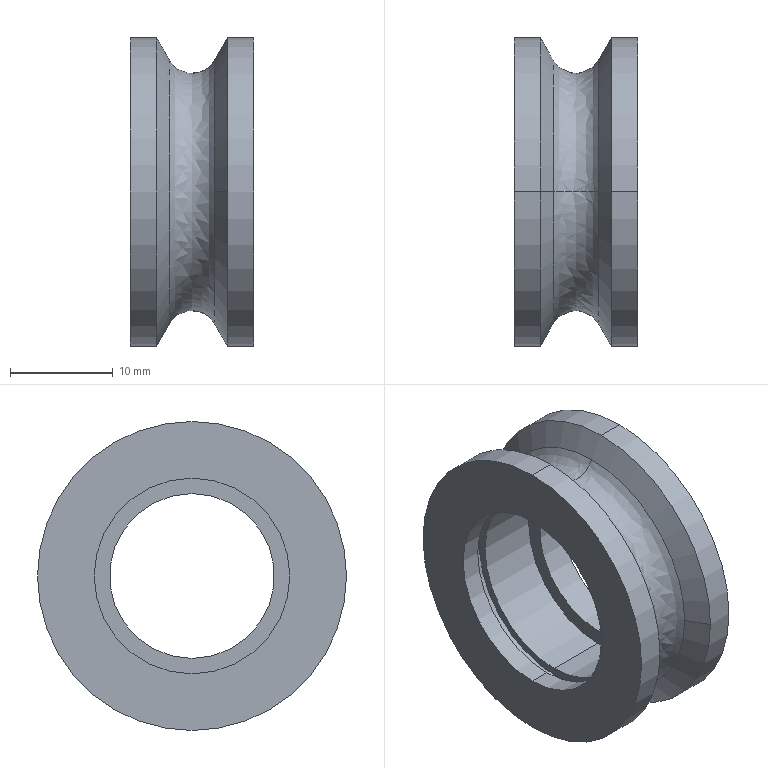Part | STEP file | _MBG28-2.5mb | 1 solid | 23 faces | box 12 x 30 x 30 mm | volume 3875 mm3 | cylinder 12 | plane 5 | cone 4 | spline 2 | commonest cylinder face diameters 19 x4 30 x4 16 x2 20.5 x2
STEP:
#1=CARTESIAN_POINT('',(3.835,0.,12.75));
#2=VERTEX_POINT('',#1);
#3=CARTESIAN_POINT('',(3.835,0.,-12.75));
#4=VERTEX_POINT('',#3);
#5=CARTESIAN_POINT('',(3.835,0.,0.));
#6=DIRECTION('',(-1.,0.,0.));
#7=DIRECTION('',(0.,0.,-1.));
#8=AXIS2_PLACEMENT_3D('',#5,#6,#7);
#9=CIRCLE('',#8,12.75);
#10=EDGE_CURVE('',#2,#4,#9,.T.);
#11=ORIENTED_EDGE('',*,*,#10,.F.);
#12=CARTESIAN_POINT('',(8.165,0.,12.75));
#13=VERTEX_POINT('',#12);
#14=CARTESIAN_POINT('',(6.,0.,14.));
#15=DIRECTION('',(0.,-1.,0.));
#16=DIRECTION('',(0.,0.,1.));
#17=AXIS2_PLACEMENT_3D('',#14,#15,#16);
#18=CIRCLE('',#17,2.5);
#19=EDGE_CURVE('',#2,#13,#18,.T.);
#20=ORIENTED_EDGE('',*,*,#19,.T.);
#21=CARTESIAN_POINT('',(8.165,12.75,0.));
#22=VERTEX_POINT('',#21);
#23=CARTESIAN_POINT('',(8.165,0.,0.));
#24=DIRECTION('',(1.,0.,0.));
#25=DIRECTION('',(0.,0.,-1.));
#26=AXIS2_PLACEMENT_3D('',#23,#24,#25);
#27=CIRCLE('',#26,12.75);
#28=EDGE_CURVE('',#22,#13,#27,.T.);
#29=ORIENTED_EDGE('',*,*,#28,.F.);
#30=CARTESIAN_POINT('',(8.165,0.,-12.75));
#31=VERTEX_POINT('',#30);
#32=CARTESIAN_POINT('',(8.165,0.,0.));
#33=DIRECTION('',(1.,0.,0.));
#34=DIRECTION('',(0.,0.,-1.));
#35=AXIS2_PLACEMENT_3D('',#32,#33,#34);
#36=CIRCLE('',#35,12.75);
#37=EDGE_CURVE('',#31,#22,#36,.T.);
#38=ORIENTED_EDGE('',*,*,#37,.F.);
#39=CARTESIAN_POINT('',(6.,0.,-14.));
#40=DIRECTION('',(0.,1.,0.));
#41=DIRECTION('',(0.,0.,-1.));
#42=AXIS2_PLACEMENT_3D('',#39,#40,#41);
#43=CIRCLE('',#42,2.5);
#44=EDGE_CURVE('',#4,#31,#43,.T.);
#45=ORIENTED_EDGE('',*,*,#44,.F.);
#46=EDGE_LOOP('',(#11,#20,#29,#38,#45));
#47=FACE_OUTER_BOUND('',#46,.T.);
#48=CARTESIAN_POINT('',(3.835,0.,-12.75));
#49=CARTESIAN_POINT('',(3.835,25.5,-12.75));
#50=CARTESIAN_POINT('',(3.835,25.5,12.75));
#51=CARTESIAN_POINT('',(3.835,0.,12.75));
#52=CARTESIAN_POINT('',(4.917,0.,-10.875));
#53=CARTESIAN_POINT('',(4.917,21.75,-10.875));
#54=CARTESIAN_POINT('',(4.917,21.75,10.875));
#55=CARTESIAN_POINT('',(4.917,0.,10.875));
#56=CARTESIAN_POINT('',(7.083,0.,-10.875));
#57=CARTESIAN_POINT('',(7.083,21.75,-10.875));
#58=CARTESIAN_POINT('',(7.083,21.75,10.875));
#59=CARTESIAN_POINT('',(7.083,0.,10.875));
#60=CARTESIAN_POINT('',(8.165,0.,-12.75));
#61=CARTESIAN_POINT('',(8.165,25.5,-12.75));
#62=CARTESIAN_POINT('',(8.165,25.5,12.75));
#63=CARTESIAN_POINT('',(8.165,0.,12.75));
#64=(BOUNDED_SURFACE()B_SPLINE_SURFACE(3,3,((#48,#49,#50,#51),(#52,#53,#54,#55),(#56,#57,#58,#59),(#60,#61,#62,#63)),.UNSPECIFIED.,.F.,.F.,.T.)B_SPLINE_SURFACE_WITH_KNOTS((4,4),(4,4),(0.,1.),(0.,1.),.UNSPECIFIED.)GEOMETRIC_REPRESENTATION_ITEM()RATIONAL_B_SPLINE_SURFACE(((1.,0.3333,0.3333,1.),(0.6667,0.2222,0.2222,0.6667),(0.6667,0.2222,0.2222,0.6667),(1.,0.3333,0.3333,1.)))REPRESENTATION_ITEM('')SURFACE());
#65=ADVANCED_FACE('',(#47),#64,.F.);
#66=CARTESIAN_POINT('',(12.,0.,-8.));
#67=VERTEX_POINT('',#66);
#68=CARTESIAN_POINT('',(12.,0.,8.));
#69=VERTEX_POINT('',#68);
#70=CARTESIAN_POINT('',(12.,0.,0.));
#71=DIRECTION('',(-1.,0.,0.));
#72=DIRECTION('',(0.,0.,1.));
#73=AXIS2_PLACEMENT_3D('',#70,#71,#72);
#74=CIRCLE('',#73,8.);
#75=EDGE_CURVE('',#67,#69,#74,.T.);
#76=ORIENTED_EDGE('',*,*,#75,.F.);
#77=CARTESIAN_POINT('',(9.,0.,-8.));
#78=VERTEX_POINT('',#77);
#79=CARTESIAN_POINT('',(12.,0.,-8.));
#80=DIRECTION('',(-1.,0.,0.));
#81=VECTOR('',#80,1000.);
#82=LINE('',#79,#81);
#83=EDGE_CURVE('',#67,#78,#82,.T.);
#84=ORIENTED_EDGE('',*,*,#83,.T.);
#85=CARTESIAN_POINT('',(9.,0.,8.));
#86=VERTEX_POINT('',#85);
#87=CARTESIAN_POINT('',(9.,0.,0.));
#88=DIRECTION('',(1.,0.,0.));
#89=DIRECTION('',(0.,0.,1.));
#90=AXIS2_PLACEMENT_3D('',#87,#88,#89);
#91=CIRCLE('',#90,8.);
#92=EDGE_CURVE('',#86,#78,#91,.T.);
#93=ORIENTED_EDGE('',*,*,#92,.F.);
#94=CARTESIAN_POINT('',(12.,0.,8.));
#95=DIRECTION('',(-1.,0.,0.));
#96=VECTOR('',#95,1000.);
#97=LINE('',#94,#96);
#98=EDGE_CURVE('',#69,#86,#97,.T.);
#99=ORIENTED_EDGE('',*,*,#98,.F.);
#100=EDGE_LOOP('',(#76,#84,#93,#99));
#101=FACE_OUTER_BOUND('',#100,.T.);
#102=CARTESIAN_POINT('',(12.,0.,0.));
#103=DIRECTION('',(-1.,0.,0.));
#104=DIRECTION('',(0.,0.,1.));
#105=AXIS2_PLACEMENT_3D('',#102,#103,#104);
#106=CYLINDRICAL_SURFACE('',#105,8.);
#107=ADVANCED_FACE('',(#101),#106,.F.);
#108=CARTESIAN_POINT('',(12.,0.,-15.));
#109=VERTEX_POINT('',#108);
#110=CARTESIAN_POINT('',(12.,0.,15.));
#111=VERTEX_POINT('',#110);
#112=CARTESIAN_POINT('',(12.,0.,0.));
#113=DIRECTION('',(1.,0.,0.));
#114=DIRECTION('',(0.,0.,1.));
#115=AXIS2_PLACEMENT_3D('',#112,#113,#114);
#116=CIRCLE('',#115,15.);
#117=EDGE_CURVE('',#109,#111,#116,.T.);
#118=ORIENTED_EDGE('',*,*,#117,.F.);
#119=CARTESIAN_POINT('',(9.464,0.,-15.));
#120=VERTEX_POINT('',#119);
#121=CARTESIAN_POINT('',(12.,0.,-15.));
#122=DIRECTION('',(-1.,0.,0.));
#123=VECTOR('',#122,1000.);
#124=LINE('',#121,#123);
#125=EDGE_CURVE('',#109,#120,#124,.T.);
#126=ORIENTED_EDGE('',*,*,#125,.T.);
#127=CARTESIAN_POINT('',(9.464,15.,0.));
#128=VERTEX_POINT('',#127);
#129=CARTESIAN_POINT('',(9.464,0.,0.));
#130=DIRECTION('',(1.,0.,0.));
#131=DIRECTION('',(0.,0.,1.));
#132=AXIS2_PLACEMENT_3D('',#129,#130,#131);
#133=CIRCLE('',#132,15.);
#134=EDGE_CURVE('',#120,#128,#133,.T.);
#135=ORIENTED_EDGE('',*,*,#134,.T.);
#136=CARTESIAN_POINT('',(9.464,0.,15.));
#137=VERTEX_POINT('',#136);
#138=CARTESIAN_POINT('',(9.464,0.,0.));
#139=DIRECTION('',(1.,0.,0.));
#140=DIRECTION('',(0.,0.,1.));
#141=AXIS2_PLACEMENT_3D('',#138,#139,#140);
#142=CIRCLE('',#141,15.);
#143=EDGE_CURVE('',#128,#137,#142,.T.);
#144=ORIENTED_EDGE('',*,*,#143,.T.);
#145=CARTESIAN_POINT('',(12.,0.,15.));
#146=DIRECTION('',(-1.,0.,0.));
#147=VECTOR('',#146,1000.);
#148=LINE('',#145,#147);
#149=EDGE_CURVE('',#111,#137,#148,.T.);
#150=ORIENTED_EDGE('',*,*,#149,.F.);
#151=EDGE_LOOP('',(#118,#126,#135,#144,#150));
#152=FACE_OUTER_BOUND('',#151,.T.);
#153=CARTESIAN_POINT('',(12.,0.,0.));
#154=DIRECTION('',(-1.,0.,0.));
#155=DIRECTION('',(0.,0.,1.));
#156=AXIS2_PLACEMENT_3D('',#153,#154,#155);
#157=CYLINDRICAL_SURFACE('',#156,15.);
#158=ADVANCED_FACE('',(#152),#157,.T.);
#159=ORIENTED_EDGE('',*,*,#28,.T.);
#160=CARTESIAN_POINT('',(8.165,-12.75,0.));
#161=VERTEX_POINT('',#160);
#162=CARTESIAN_POINT('',(8.165,0.,0.));
#163=DIRECTION('',(1.,0.,0.));
#164=DIRECTION('',(0.,0.,-1.));
#165=AXIS2_PLACEMENT_3D('',#162,#163,#164);
#166=CIRCLE('',#165,12.75);
#167=EDGE_CURVE('',#13,#161,#166,.T.);
#168=ORIENTED_EDGE('',*,*,#167,.T.);
#169=CARTESIAN_POINT('',(9.464,-15.,0.));
#170=VERTEX_POINT('',#169);
#171=CARTESIAN_POINT('',(9.464,-15.,0.));
#172=DIRECTION('',(0.5,-0.866,0.));
#173=VECTOR('',#172,1000.);
#174=LINE('',#171,#173);
#175=EDGE_CURVE('',#161,#170,#174,.T.);
#176=ORIENTED_EDGE('',*,*,#175,.T.);
#177=CARTESIAN_POINT('',(9.464,0.,0.));
#178=DIRECTION('',(1.,0.,0.));
#179=DIRECTION('',(0.,0.,1.));
#180=AXIS2_PLACEMENT_3D('',#177,#178,#179);
#181=CIRCLE('',#180,15.);
#182=EDGE_CURVE('',#137,#170,#181,.T.);
#183=ORIENTED_EDGE('',*,*,#182,.F.);
#184=ORIENTED_EDGE('',*,*,#143,.F.);
#185=CARTESIAN_POINT('',(9.464,15.,0.));
#186=DIRECTION('',(0.5,0.866,0.));
#187=VECTOR('',#186,1000.);
#188=LINE('',#185,#187);
#189=EDGE_CURVE('',#22,#128,#188,.T.);
#190=ORIENTED_EDGE('',*,*,#189,.F.);
#191=EDGE_LOOP('',(#159,#168,#176,#183,#184,#190));
#192=FACE_OUTER_BOUND('',#191,.T.);
#193=CARTESIAN_POINT('',(9.464,0.,0.));
#194=DIRECTION('',(1.,0.,0.));
#195=DIRECTION('',(0.,1.,0.));
#196=AXIS2_PLACEMENT_3D('',#193,#194,#195);
#197=CONICAL_SURFACE('',#196,15.,1.047);
#198=ADVANCED_FACE('',(#192),#197,.T.);
#199=CARTESIAN_POINT('',(9.,0.,-9.5));
#200=VERTEX_POINT('',#199);
#201=CARTESIAN_POINT('',(9.,0.,9.5));
#202=VERTEX_POINT('',#201);
#203=CARTESIAN_POINT('',(9.,0.,0.));
#204=DIRECTION('',(-1.,0.,0.));
#205=DIRECTION('',(0.,0.,1.));
#206=AXIS2_PLACEMENT_3D('',#203,#204,#205);
#207=CIRCLE('',#206,9.5);
#208=EDGE_CURVE('',#200,#202,#207,.T.);
#209=ORIENTED_EDGE('',*,*,#208,.F.);
#210=CARTESIAN_POINT('',(3.,0.,-9.5));
#211=VERTEX_POINT('',#210);
#212=CARTESIAN_POINT('',(12.,0.,-9.5));
#213=DIRECTION('',(-1.,0.,0.));
#214=VECTOR('',#213,1000.);
#215=LINE('',#212,#214);
#216=EDGE_CURVE('',#200,#211,#215,.T.);
#217=ORIENTED_EDGE('',*,*,#216,.T.);
#218=CARTESIAN_POINT('',(3.,0.,9.5));
#219=VERTEX_POINT('',#218);
#220=CARTESIAN_POINT('',(3.,0.,0.));
#221=DIRECTION('',(1.,0.,0.));
#222=DIRECTION('',(0.,0.,1.));
#223=AXIS2_PLACEMENT_3D('',#220,#221,#222);
#224=CIRCLE('',#223,9.5);
#225=EDGE_CURVE('',#219,#211,#224,.T.);
#226=ORIENTED_EDGE('',*,*,#225,.F.);
#227=CARTESIAN_POINT('',(12.,0.,9.5));
#228=DIRECTION('',(-1.,0.,0.));
#229=VECTOR('',#228,1000.);
#230=LINE('',#227,#229);
#231=EDGE_CURVE('',#202,#219,#230,.T.);
#232=ORIENTED_EDGE('',*,*,#231,.F.);
#233=EDGE_LOOP('',(#209,#217,#226,#232));
#234=FACE_OUTER_BOUND('',#233,.T.);
#235=CARTESIAN_POINT('',(12.,0.,0.));
#236=DIRECTION('',(-1.,0.,0.));
#237=DIRECTION('',(0.,0.,1.));
#238=AXIS2_PLACEMENT_3D('',#235,#236,#237);
#239=CYLINDRICAL_SURFACE('',#238,9.5);
#240=ADVANCED_FACE('',(#234),#239,.F.);
#241=ORIENTED_EDGE('',*,*,#10,.T.);
#242=CARTESIAN_POINT('',(2.536,0.,-15.));
#243=VERTEX_POINT('',#242);
#244=CARTESIAN_POINT('',(2.536,0.,-15.));
#245=DIRECTION('',(-0.5,0.,-0.866));
#246=VECTOR('',#245,1000.);
#247=LINE('',#244,#246);
#248=EDGE_CURVE('',#4,#243,#247,.T.);
#249=ORIENTED_EDGE('',*,*,#248,.T.);
#250=CARTESIAN_POINT('',(2.536,0.,15.));
#251=VERTEX_POINT('',#250);
#252=CARTESIAN_POINT('',(2.536,0.,0.));
#253=DIRECTION('',(1.,0.,0.));
#254=DIRECTION('',(0.,0.,1.));
#255=AXIS2_PLACEMENT_3D('',#252,#253,#254);
#256=CIRCLE('',#255,15.);
#257=EDGE_CURVE('',#243,#251,#256,.T.);
#258=ORIENTED_EDGE('',*,*,#257,.T.);
#259=CARTESIAN_POINT('',(2.536,0.,15.));
#260=DIRECTION('',(-0.5,0.,0.866));
#261=VECTOR('',#260,1000.);
#262=LINE('',#259,#261);
#263=EDGE_CURVE('',#2,#251,#262,.T.);
#264=ORIENTED_EDGE('',*,*,#263,.F.);
#265=EDGE_LOOP('',(#241,#249,#258,#264));
#266=FACE_OUTER_BOUND('',#265,.T.);
#267=CARTESIAN_POINT('',(2.536,0.,0.));
#268=DIRECTION('',(-1.,0.,0.));
#269=DIRECTION('',(0.,0.,1.));
#270=AXIS2_PLACEMENT_3D('',#267,#268,#269);
#271=CONICAL_SURFACE('',#270,15.,1.047);
#272=ADVANCED_FACE('',(#266),#271,.T.);
#273=CARTESIAN_POINT('',(3.,0.,-10.25));
#274=VERTEX_POINT('',#273);
#275=CARTESIAN_POINT('',(3.,0.,10.25));
#276=VERTEX_POINT('',#275);
#277=CARTESIAN_POINT('',(3.,0.,0.));
#278=DIRECTION('',(-1.,0.,0.));
#279=DIRECTION('',(0.,0.,1.));
#280=AXIS2_PLACEMENT_3D('',#277,#278,#279);
#281=CIRCLE('',#280,10.25);
#282=EDGE_CURVE('',#274,#276,#281,.T.);
#283=ORIENTED_EDGE('',*,*,#282,.F.);
#284=CARTESIAN_POINT('',(2.,0.,-10.25));
#285=VERTEX_POINT('',#284);
#286=CARTESIAN_POINT('',(12.,0.,-10.25));
#287=DIRECTION('',(-1.,0.,0.));
#288=VECTOR('',#287,1000.);
#289=LINE('',#286,#288);
#290=EDGE_CURVE('',#274,#285,#289,.T.);
#291=ORIENTED_EDGE('',*,*,#290,.T.);
#292=CARTESIAN_POINT('',(2.,0.,10.25));
#293=VERTEX_POINT('',#292);
#294=CARTESIAN_POINT('',(2.,0.,0.));
#295=DIRECTION('',(1.,0.,0.));
#296=DIRECTION('',(0.,0.,1.));
#297=AXIS2_PLACEMENT_3D('',#294,#295,#296);
#298=CIRCLE('',#297,10.25);
#299=EDGE_CURVE('',#293,#285,#298,.T.);
#300=ORIENTED_EDGE('',*,*,#299,.F.);
#301=CARTESIAN_POINT('',(12.,0.,10.25));
#302=DIRECTION('',(-1.,0.,0.));
#303=VECTOR('',#302,1000.);
#304=LINE('',#301,#303);
#305=EDGE_CURVE('',#276,#293,#304,.T.);
#306=ORIENTED_EDGE('',*,*,#305,.F.);
#307=EDGE_LOOP('',(#283,#291,#300,#306));
#308=FACE_OUTER_BOUND('',#307,.T.);
#309=CARTESIAN_POINT('',(12.,0.,0.));
#310=DIRECTION('',(-1.,0.,0.));
#311=DIRECTION('',(0.,0.,1.));
#312=AXIS2_PLACEMENT_3D('',#309,#310,#311);
#313=CYLINDRICAL_SURFACE('',#312,10.25);
#314=ADVANCED_FACE('',(#308),#313,.F.);
#315=ORIENTED_EDGE('',*,*,#257,.F.);
#316=CARTESIAN_POINT('',(0.,0.,-15.));
#317=VERTEX_POINT('',#316);
#318=CARTESIAN_POINT('',(12.,0.,-15.));
#319=DIRECTION('',(-1.,0.,0.));
#320=VECTOR('',#319,1000.);
#321=LINE('',#318,#320);
#322=EDGE_CURVE('',#243,#317,#321,.T.);
#323=ORIENTED_EDGE('',*,*,#322,.T.);
#324=CARTESIAN_POINT('',(0.,0.,15.));
#325=VERTEX_POINT('',#324);
#326=CARTESIAN_POINT('',(0.,0.,0.));
#327=DIRECTION('',(1.,0.,0.));
#328=DIRECTION('',(0.,0.,1.));
#329=AXIS2_PLACEMENT_3D('',#326,#327,#328);
#330=CIRCLE('',#329,15.);
#331=EDGE_CURVE('',#317,#325,#330,.T.);
#332=ORIENTED_EDGE('',*,*,#331,.T.);
#333=CARTESIAN_POINT('',(12.,0.,15.));
#334=DIRECTION('',(-1.,0.,0.));
#335=VECTOR('',#334,1000.);
#336=LINE('',#333,#335);
#337=EDGE_CURVE('',#251,#325,#336,.T.);
#338=ORIENTED_EDGE('',*,*,#337,.F.);
#339=EDGE_LOOP('',(#315,#323,#332,#338));
#340=FACE_OUTER_BOUND('',#339,.T.);
#341=CARTESIAN_POINT('',(12.,0.,0.));
#342=DIRECTION('',(-1.,0.,0.));
#343=DIRECTION('',(0.,0.,1.));
#344=AXIS2_PLACEMENT_3D('',#341,#342,#343);
#345=CYLINDRICAL_SURFACE('',#344,15.);
#346=ADVANCED_FACE('',(#340),#345,.T.);
#347=CARTESIAN_POINT('',(2.,0.,-9.5));
#348=VERTEX_POINT('',#347);
#349=CARTESIAN_POINT('',(2.,0.,9.5));
#350=VERTEX_POINT('',#349);
#351=CARTESIAN_POINT('',(2.,0.,0.));
#352=DIRECTION('',(-1.,0.,0.));
#353=DIRECTION('',(0.,0.,1.));
#354=AXIS2_PLACEMENT_3D('',#351,#352,#353);
#355=CIRCLE('',#354,9.5);
#356=EDGE_CURVE('',#348,#350,#355,.T.);
#357=ORIENTED_EDGE('',*,*,#356,.F.);
#358=CARTESIAN_POINT('',(0.,0.,-9.5));
#359=VERTEX_POINT('',#358);
#360=CARTESIAN_POINT('',(12.,0.,-9.5));
#361=DIRECTION('',(-1.,0.,0.));
#362=VECTOR('',#361,1000.);
#363=LINE('',#360,#362);
#364=EDGE_CURVE('',#348,#359,#363,.T.);
#365=ORIENTED_EDGE('',*,*,#364,.T.);
#366=CARTESIAN_POINT('',(0.,0.,9.5));
#367=VERTEX_POINT('',#366);
#368=CARTESIAN_POINT('',(0.,0.,0.));
#369=DIRECTION('',(1.,0.,0.));
#370=DIRECTION('',(0.,0.,1.));
#371=AXIS2_PLACEMENT_3D('',#368,#369,#370);
#372=CIRCLE('',#371,9.5);
#373=EDGE_CURVE('',#367,#359,#372,.T.);
#374=ORIENTED_EDGE('',*,*,#373,.F.);
#375=CARTESIAN_POINT('',(12.,0.,9.5));
#376=DIRECTION('',(-1.,0.,0.));
#377=VECTOR('',#376,1000.);
#378=LINE('',#375,#377);
#379=EDGE_CURVE('',#350,#367,#378,.T.);
#380=ORIENTED_EDGE('',*,*,#379,.F.);
#381=EDGE_LOOP('',(#357,#365,#374,#380));
#382=FACE_OUTER_BOUND('',#381,.T.);
#383=CARTESIAN_POINT('',(12.,0.,0.));
#384=DIRECTION('',(-1.,0.,0.));
#385=DIRECTION('',(0.,0.,1.));
#386=AXIS2_PLACEMENT_3D('',#383,#384,#385);
#387=CYLINDRICAL_SURFACE('',#386,9.5);
#388=ADVANCED_FACE('',(#382),#387,.F.);
#389=CARTESIAN_POINT('',(12.,0.,0.));
#390=DIRECTION('',(-1.,0.,0.));
#391=DIRECTION('',(0.,0.,1.));
#392=AXIS2_PLACEMENT_3D('',#389,#390,#391);
#393=CIRCLE('',#392,8.);
#394=EDGE_CURVE('',#69,#67,#393,.T.);
#395=ORIENTED_EDGE('',*,*,#394,.T.);
#396=ORIENTED_EDGE('',*,*,#75,.T.);
#397=EDGE_LOOP('',(#395,#396));
#398=FACE_BOUND('',#397,.T.);
#399=CARTESIAN_POINT('',(12.,0.,0.));
#400=DIRECTION('',(1.,0.,0.));
#401=DIRECTION('',(0.,0.,1.));
#402=AXIS2_PLACEMENT_3D('',#399,#400,#401);
#403=CIRCLE('',#402,15.);
#404=EDGE_CURVE('',#111,#109,#403,.T.);
#405=ORIENTED_EDGE('',*,*,#404,.T.);
#406=ORIENTED_EDGE('',*,*,#117,.T.);
#407=EDGE_LOOP('',(#405,#406));
#408=FACE_OUTER_BOUND('',#407,.T.);
#409=CARTESIAN_POINT('',(12.,8.,0.));
#410=DIRECTION('',(1.,0.,0.));
#411=DIRECTION('',(0.,0.,-1.));
#412=AXIS2_PLACEMENT_3D('',#409,#410,#411);
#413=PLANE('',#412);
#414=ADVANCED_FACE('',(#398,#408),#413,.T.);
#415=ORIENTED_EDGE('',*,*,#83,.F.);
#416=ORIENTED_EDGE('',*,*,#394,.F.);
#417=ORIENTED_EDGE('',*,*,#98,.T.);
#418=CARTESIAN_POINT('',(9.,0.,0.));
#419=DIRECTION('',(1.,0.,0.));
#420=DIRECTION('',(0.,0.,1.));
#421=AXIS2_PLACEMENT_3D('',#418,#419,#420);
#422=CIRCLE('',#421,8.);
#423=EDGE_CURVE('',#78,#86,#422,.T.);
#424=ORIENTED_EDGE('',*,*,#423,.F.);
#425=EDGE_LOOP('',(#415,#416,#417,#424));
#426=FACE_OUTER_BOUND('',#425,.T.);
#427=CARTESIAN_POINT('',(12.,0.,0.));
#428=DIRECTION('',(-1.,0.,0.));
#429=DIRECTION('',(0.,0.,1.));
#430=AXIS2_PLACEMENT_3D('',#427,#428,#429);
#431=CYLINDRICAL_SURFACE('',#430,8.);
#432=ADVANCED_FACE('',(#426),#431,.F.);
#433=ORIENTED_EDGE('',*,*,#125,.F.);
#434=ORIENTED_EDGE('',*,*,#404,.F.);
#435=ORIENTED_EDGE('',*,*,#149,.T.);
#436=ORIENTED_EDGE('',*,*,#182,.T.);
#437=CARTESIAN_POINT('',(9.464,0.,0.));
#438=DIRECTION('',(1.,0.,0.));
#439=DIRECTION('',(0.,0.,1.));
#440=AXIS2_PLACEMENT_3D('',#437,#438,#439);
#441=CIRCLE('',#440,15.);
#442=EDGE_CURVE('',#170,#120,#441,.T.);
#443=ORIENTED_EDGE('',*,*,#442,.T.);
#444=EDGE_LOOP('',(#433,#434,#435,#436,#443));
#445=FACE_OUTER_BOUND('',#444,.T.);
#446=CARTESIAN_POINT('',(12.,0.,0.));
#447=DIRECTION('',(-1.,0.,0.));
#448=DIRECTION('',(0.,0.,1.));
#449=AXIS2_PLACEMENT_3D('',#446,#447,#448);
#450=CYLINDRICAL_SURFACE('',#449,15.);
#451=ADVANCED_FACE('',(#445),#450,.T.);
#452=CARTESIAN_POINT('',(9.,0.,0.));
#453=DIRECTION('',(-1.,0.,0.));
#454=DIRECTION('',(0.,0.,1.));
#455=AXIS2_PLACEMENT_3D('',#452,#453,#454);
#456=CIRCLE('',#455,9.5);
#457=EDGE_CURVE('',#202,#200,#456,.T.);
#458=ORIENTED_EDGE('',*,*,#457,.T.);
#459=ORIENTED_EDGE('',*,*,#208,.T.);
#460=EDGE_LOOP('',(#458,#459));
#461=FACE_OUTER_BOUND('',#460,.T.);
#462=ORIENTED_EDGE('',*,*,#92,.T.);
#463=ORIENTED_EDGE('',*,*,#423,.T.);
#464=EDGE_LOOP('',(#462,#463));
#465=FACE_BOUND('',#464,.T.);
#466=CARTESIAN_POINT('',(9.,9.5,0.));
#467=DIRECTION('',(-1.,0.,0.));
#468=DIRECTION('',(0.,0.,1.));
#469=AXIS2_PLACEMENT_3D('',#466,#467,#468);
#470=PLANE('',#469);
#471=ADVANCED_FACE('',(#461,#465),#470,.T.);
#472=ORIENTED_EDGE('',*,*,#175,.F.);
#473=CARTESIAN_POINT('',(8.165,0.,0.));
#474=DIRECTION('',(1.,0.,0.));
#475=DIRECTION('',(0.,0.,-1.));
#476=AXIS2_PLACEMENT_3D('',#473,#474,#475);
#477=CIRCLE('',#476,12.75);
#478=EDGE_CURVE('',#161,#31,#477,.T.);
#479=ORIENTED_EDGE('',*,*,#478,.T.);
#480=ORIENTED_EDGE('',*,*,#37,.T.);
#481=ORIENTED_EDGE('',*,*,#189,.T.);
#482=ORIENTED_EDGE('',*,*,#134,.F.);
#483=ORIENTED_EDGE('',*,*,#442,.F.);
#484=EDGE_LOOP('',(#472,#479,#480,#481,#482,#483));
#485=FACE_OUTER_BOUND('',#484,.T.);
#486=CARTESIAN_POINT('',(9.464,0.,0.));
#487=DIRECTION('',(1.,0.,0.));
#488=DIRECTION('',(0.,1.,0.));
#489=AXIS2_PLACEMENT_3D('',#486,#487,#488);
#490=CONICAL_SURFACE('',#489,15.,1.047);
#491=ADVANCED_FACE('',(#485),#490,.T.);
#492=ORIENTED_EDGE('',*,*,#216,.F.);
#493=ORIENTED_EDGE('',*,*,#457,.F.);
#494=ORIENTED_EDGE('',*,*,#231,.T.);
#495=CARTESIAN_POINT('',(3.,0.,0.));
#496=DIRECTION('',(1.,0.,0.));
#497=DIRECTION('',(0.,0.,1.));
#498=AXIS2_PLACEMENT_3D('',#495,#496,#497);
#499=CIRCLE('',#498,9.5);
#500=EDGE_CURVE('',#211,#219,#499,.T.);
#501=ORIENTED_EDGE('',*,*,#500,.F.);
#502=EDGE_LOOP('',(#492,#493,#494,#501));
#503=FACE_OUTER_BOUND('',#502,.T.);
#504=CARTESIAN_POINT('',(12.,0.,0.));
#505=DIRECTION('',(-1.,0.,0.));
#506=DIRECTION('',(0.,0.,1.));
#507=AXIS2_PLACEMENT_3D('',#504,#505,#506);
#508=CYLINDRICAL_SURFACE('',#507,9.5);
#509=ADVANCED_FACE('',(#503),#508,.F.);
#510=ORIENTED_EDGE('',*,*,#19,.F.);
#511=CARTESIAN_POINT('',(3.835,0.,0.));
#512=DIRECTION('',(-1.,0.,0.));
#513=DIRECTION('',(0.,0.,-1.));
#514=AXIS2_PLACEMENT_3D('',#511,#512,#513);
#515=CIRCLE('',#514,12.75);
#516=EDGE_CURVE('',#4,#2,#515,.T.);
#517=ORIENTED_EDGE('',*,*,#516,.F.);
#518=ORIENTED_EDGE('',*,*,#44,.T.);
#519=ORIENTED_EDGE('',*,*,#478,.F.);
#520=ORIENTED_EDGE('',*,*,#167,.F.);
#521=EDGE_LOOP('',(#510,#517,#518,#519,#520));
#522=FACE_OUTER_BOUND('',#521,.T.);
#523=CARTESIAN_POINT('',(3.835,0.,12.75));
#524=CARTESIAN_POINT('',(3.835,-25.5,12.75));
#525=CARTESIAN_POINT('',(3.835,-25.5,-12.75));
#526=CARTESIAN_POINT('',(3.835,0.,-12.75));
#527=CARTESIAN_POINT('',(4.917,0.,10.875));
#528=CARTESIAN_POINT('',(4.917,-21.75,10.875));
#529=CARTESIAN_POINT('',(4.917,-21.75,-10.875));
#530=CARTESIAN_POINT('',(4.917,0.,-10.875));
#531=CARTESIAN_POINT('',(7.083,0.,10.875));
#532=CARTESIAN_POINT('',(7.083,-21.75,10.875));
#533=CARTESIAN_POINT('',(7.083,-21.75,-10.875));
#534=CARTESIAN_POINT('',(7.083,0.,-10.875));
#535=CARTESIAN_POINT('',(8.165,0.,12.75));
#536=CARTESIAN_POINT('',(8.165,-25.5,12.75));
#537=CARTESIAN_POINT('',(8.165,-25.5,-12.75));
#538=CARTESIAN_POINT('',(8.165,0.,-12.75));
#539=(BOUNDED_SURFACE()B_SPLINE_SURFACE(3,3,((#523,#524,#525,#526),(#527,#528,#529,#530),(#531,#532,#533,#534),(#535,#536,#537,#538)),.UNSPECIFIED.,.F.,.F.,.T.)B_SPLINE_SURFACE_WITH_KNOTS((4,4),(4,4),(0.,1.),(0.,1.),.UNSPECIFIED.)GEOMETRIC_REPRESENTATION_ITEM()RATIONAL_B_SPLINE_SURFACE(((1.,0.3333,0.3333,1.),(0.6667,0.2222,0.2222,0.6667),(0.6667,0.2222,0.2222,0.6667),(1.,0.3333,0.3333,1.)))REPRESENTATION_ITEM('')SURFACE());
#540=ADVANCED_FACE('',(#522),#539,.F.);
#541=CARTESIAN_POINT('',(3.,0.,0.));
#542=DIRECTION('',(-1.,0.,0.));
#543=DIRECTION('',(0.,0.,1.));
#544=AXIS2_PLACEMENT_3D('',#541,#542,#543);
#545=CIRCLE('',#544,10.25);
#546=EDGE_CURVE('',#276,#274,#545,.T.);
#547=ORIENTED_EDGE('',*,*,#546,.T.);
#548=ORIENTED_EDGE('',*,*,#282,.T.);
#549=EDGE_LOOP('',(#547,#548));
#550=FACE_OUTER_BOUND('',#549,.T.);
#551=ORIENTED_EDGE('',*,*,#225,.T.);
#552=ORIENTED_EDGE('',*,*,#500,.T.);
#553=EDGE_LOOP('',(#551,#552));
#554=FACE_BOUND('',#553,.T.);
#555=CARTESIAN_POINT('',(3.,10.25,0.));
#556=DIRECTION('',(-1.,0.,0.));
#557=DIRECTION('',(0.,0.,1.));
#558=AXIS2_PLACEMENT_3D('',#555,#556,#557);
#559=PLANE('',#558);
#560=ADVANCED_FACE('',(#550,#554),#559,.T.);
#561=ORIENTED_EDGE('',*,*,#248,.F.);
#562=ORIENTED_EDGE('',*,*,#516,.T.);
#563=ORIENTED_EDGE('',*,*,#263,.T.);
#564=CARTESIAN_POINT('',(2.536,0.,0.));
#565=DIRECTION('',(1.,0.,0.));
#566=DIRECTION('',(0.,0.,1.));
#567=AXIS2_PLACEMENT_3D('',#564,#565,#566);
#568=CIRCLE('',#567,15.);
#569=EDGE_CURVE('',#251,#243,#568,.T.);
#570=ORIENTED_EDGE('',*,*,#569,.T.);
#571=EDGE_LOOP('',(#561,#562,#563,#570));
#572=FACE_OUTER_BOUND('',#571,.T.);
#573=CARTESIAN_POINT('',(2.536,0.,0.));
#574=DIRECTION('',(-1.,0.,0.));
#575=DIRECTION('',(0.,0.,1.));
#576=AXIS2_PLACEMENT_3D('',#573,#574,#575);
#577=CONICAL_SURFACE('',#576,15.,1.047);
#578=ADVANCED_FACE('',(#572),#577,.T.);
#579=ORIENTED_EDGE('',*,*,#290,.F.);
#580=ORIENTED_EDGE('',*,*,#546,.F.);
#581=ORIENTED_EDGE('',*,*,#305,.T.);
#582=CARTESIAN_POINT('',(2.,0.,0.));
#583=DIRECTION('',(1.,0.,0.));
#584=DIRECTION('',(0.,0.,1.));
#585=AXIS2_PLACEMENT_3D('',#582,#583,#584);
#586=CIRCLE('',#585,10.25);
#587=EDGE_CURVE('',#285,#293,#586,.T.);
#588=ORIENTED_EDGE('',*,*,#587,.F.);
#589=EDGE_LOOP('',(#579,#580,#581,#588));
#590=FACE_OUTER_BOUND('',#589,.T.);
#591=CARTESIAN_POINT('',(12.,0.,0.));
#592=DIRECTION('',(-1.,0.,0.));
#593=DIRECTION('',(0.,0.,1.));
#594=AXIS2_PLACEMENT_3D('',#591,#592,#593);
#595=CYLINDRICAL_SURFACE('',#594,10.25);
#596=ADVANCED_FACE('',(#590),#595,.F.);
#597=ORIENTED_EDGE('',*,*,#322,.F.);
#598=ORIENTED_EDGE('',*,*,#569,.F.);
#599=ORIENTED_EDGE('',*,*,#337,.T.);
#600=CARTESIAN_POINT('',(0.,0.,0.));
#601=DIRECTION('',(1.,0.,0.));
#602=DIRECTION('',(0.,0.,1.));
#603=AXIS2_PLACEMENT_3D('',#600,#601,#602);
#604=CIRCLE('',#603,15.);
#605=EDGE_CURVE('',#325,#317,#604,.T.);
#606=ORIENTED_EDGE('',*,*,#605,.T.);
#607=EDGE_LOOP('',(#597,#598,#599,#606));
#608=FACE_OUTER_BOUND('',#607,.T.);
#609=CARTESIAN_POINT('',(12.,0.,0.));
#610=DIRECTION('',(-1.,0.,0.));
#611=DIRECTION('',(0.,0.,1.));
#612=AXIS2_PLACEMENT_3D('',#609,#610,#611);
#613=CYLINDRICAL_SURFACE('',#612,15.);
#614=ADVANCED_FACE('',(#608),#613,.T.);
#615=CARTESIAN_POINT('',(2.,0.,0.));
#616=DIRECTION('',(-1.,0.,0.));
#617=DIRECTION('',(0.,0.,1.));
#618=AXIS2_PLACEMENT_3D('',#615,#616,#617);
#619=CIRCLE('',#618,9.5);
#620=EDGE_CURVE('',#350,#348,#619,.T.);
#621=ORIENTED_EDGE('',*,*,#620,.T.);
#622=ORIENTED_EDGE('',*,*,#356,.T.);
#623=EDGE_LOOP('',(#621,#622));
#624=FACE_BOUND('',#623,.T.);
#625=ORIENTED_EDGE('',*,*,#299,.T.);
#626=ORIENTED_EDGE('',*,*,#587,.T.);
#627=EDGE_LOOP('',(#625,#626));
#628=FACE_OUTER_BOUND('',#627,.T.);
#629=CARTESIAN_POINT('',(2.,9.5,0.));
#630=DIRECTION('',(1.,0.,0.));
#631=DIRECTION('',(0.,0.,-1.));
#632=AXIS2_PLACEMENT_3D('',#629,#630,#631);
#633=PLANE('',#632);
#634=ADVANCED_FACE('',(#624,#628),#633,.T.);
#635=ORIENTED_EDGE('',*,*,#605,.F.);
#636=ORIENTED_EDGE('',*,*,#331,.F.);
#637=EDGE_LOOP('',(#635,#636));
#638=FACE_OUTER_BOUND('',#637,.T.);
#639=ORIENTED_EDGE('',*,*,#373,.T.);
#640=CARTESIAN_POINT('',(0.,0.,0.));
#641=DIRECTION('',(1.,0.,0.));
#642=DIRECTION('',(0.,0.,1.));
#643=AXIS2_PLACEMENT_3D('',#640,#641,#642);
#644=CIRCLE('',#643,9.5);
#645=EDGE_CURVE('',#359,#367,#644,.T.);
#646=ORIENTED_EDGE('',*,*,#645,.T.);
#647=EDGE_LOOP('',(#639,#646));
#648=FACE_BOUND('',#647,.T.);
#649=CARTESIAN_POINT('',(0.,15.,0.));
#650=DIRECTION('',(-1.,0.,0.));
#651=DIRECTION('',(0.,0.,1.));
#652=AXIS2_PLACEMENT_3D('',#649,#650,#651);
#653=PLANE('',#652);
#654=ADVANCED_FACE('',(#638,#648),#653,.T.);
#655=ORIENTED_EDGE('',*,*,#364,.F.);
#656=ORIENTED_EDGE('',*,*,#620,.F.);
#657=ORIENTED_EDGE('',*,*,#379,.T.);
#658=ORIENTED_EDGE('',*,*,#645,.F.);
#659=EDGE_LOOP('',(#655,#656,#657,#658));
#660=FACE_OUTER_BOUND('',#659,.T.);
#661=CARTESIAN_POINT('',(12.,0.,0.));
#662=DIRECTION('',(-1.,0.,0.));
#663=DIRECTION('',(0.,0.,1.));
#664=AXIS2_PLACEMENT_3D('',#661,#662,#663);
#665=CYLINDRICAL_SURFACE('',#664,9.5);
#666=ADVANCED_FACE('',(#660),#665,.F.);
#667=CLOSED_SHELL('',(#65,#107,#158,#198,#240,#272,#314,#346,#388,#414,#432,#451,#471,#491,#509,#540,#560,#578,#596,#614,#634,#654,#666));
#668=MANIFOLD_SOLID_BREP('',#667);
#669=CARTESIAN_POINT('',(0.,0.,0.));
#670=DIRECTION('',(0.,0.,1.));
#671=DIRECTION('',(1.,0.,0.));
#672=AXIS2_PLACEMENT_3D('',#669,#670,#671);
#673=(LENGTH_UNIT()NAMED_UNIT(*)SI_UNIT(.MILLI.,.METRE.));
#674=UNCERTAINTY_MEASURE_WITH_UNIT(LENGTH_MEASURE(0.00001),#673,'','');
#675=(NAMED_UNIT(*)PLANE_ANGLE_UNIT()SI_UNIT($,.RADIAN.));
#676=(NAMED_UNIT(*)SI_UNIT($,.STERADIAN.)SOLID_ANGLE_UNIT());
#677=(GEOMETRIC_REPRESENTATION_CONTEXT(3)GLOBAL_UNCERTAINTY_ASSIGNED_CONTEXT((#674))GLOBAL_UNIT_ASSIGNED_CONTEXT((#673,#675,#676))REPRESENTATION_CONTEXT('',''));
#678=ADVANCED_BREP_SHAPE_REPRESENTATION('',(#668,#672),#677);